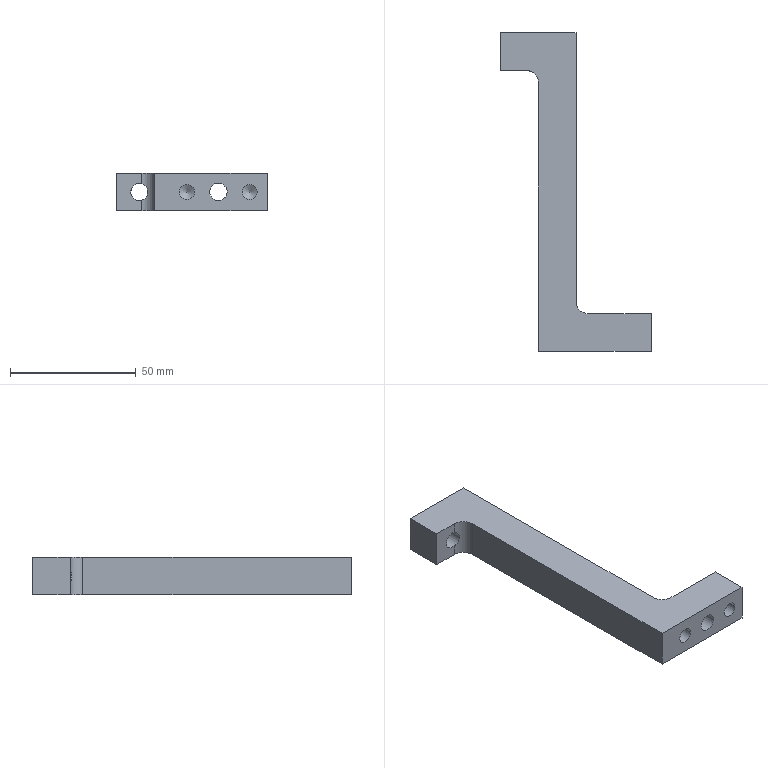Part | NX | features BREP 1 | 1 solid | 18 faces | box 60 x 127 x 15 mm | volume 37025 mm3 | plane 10 | cylinder 6 | cone 2 | commonest cylinder face diameters 6 x2 10 x2 6.8 x1 7 x1
STEP:
#1=CARTESIAN_POINT('',(14.,0.,7.5));
#2=VERTEX_POINT('',#1);
#3=CARTESIAN_POINT('',(10.5,0.,7.5));
#4=DIRECTION('',(0.,-1.,0.));
#5=DIRECTION('',(1.,0.,0.));
#6=AXIS2_PLACEMENT_3D('',#3,#4,#5);
#7=CIRCLE('',#6,3.5);
#8=EDGE_CURVE('',#2,#2,#7,.T.);
#9=ORIENTED_EDGE('',*,*,#8,.T.);
#10=EDGE_LOOP('',(#9));
#11=FACE_BOUND('',#10,.T.);
#12=CARTESIAN_POINT('',(30.,0.,0.));
#13=VERTEX_POINT('',#12);
#14=CARTESIAN_POINT('',(5.,0.,0.));
#15=VERTEX_POINT('',#14);
#16=CARTESIAN_POINT('',(30.,0.,0.));
#17=DIRECTION('',(-1.,0.,0.));
#18=VECTOR('',#17,1000.);
#19=LINE('',#16,#18);
#20=EDGE_CURVE('',#13,#15,#19,.T.);
#21=ORIENTED_EDGE('',*,*,#20,.T.);
#22=CARTESIAN_POINT('',(5.,0.,15.));
#23=VERTEX_POINT('',#22);
#24=CARTESIAN_POINT('',(5.,0.,15.));
#25=DIRECTION('',(0.,0.,1.));
#26=VECTOR('',#25,1000.);
#27=LINE('',#24,#26);
#28=EDGE_CURVE('',#15,#23,#27,.T.);
#29=ORIENTED_EDGE('',*,*,#28,.T.);
#30=CARTESIAN_POINT('',(30.,0.,15.));
#31=VERTEX_POINT('',#30);
#32=CARTESIAN_POINT('',(30.,0.,15.));
#33=DIRECTION('',(-1.,0.,0.));
#34=VECTOR('',#33,1000.);
#35=LINE('',#32,#34);
#36=EDGE_CURVE('',#31,#23,#35,.T.);
#37=ORIENTED_EDGE('',*,*,#36,.F.);
#38=CARTESIAN_POINT('',(30.,0.,15.));
#39=DIRECTION('',(0.,0.,-1.));
#40=VECTOR('',#39,1000.);
#41=LINE('',#38,#40);
#42=EDGE_CURVE('',#31,#13,#41,.T.);
#43=ORIENTED_EDGE('',*,*,#42,.T.);
#44=EDGE_LOOP('',(#21,#29,#37,#43));
#45=FACE_BOUND('',#44,.T.);
#46=CARTESIAN_POINT('',(30.,0.,15.));
#47=DIRECTION('',(0.,-1.,0.));
#48=DIRECTION('',(-1.,0.,0.));
#49=AXIS2_PLACEMENT_3D('',#46,#47,#48);
#50=PLANE('',#49);
#51=ADVANCED_FACE('',(#11,#45),#50,.F.);
#52=CARTESIAN_POINT('',(0.,5.,15.));
#53=VERTEX_POINT('',#52);
#54=CARTESIAN_POINT('',(0.,112.,15.));
#55=VERTEX_POINT('',#54);
#56=CARTESIAN_POINT('',(0.,0.,15.));
#57=DIRECTION('',(0.,1.,0.));
#58=VECTOR('',#57,1000.);
#59=LINE('',#56,#58);
#60=EDGE_CURVE('',#53,#55,#59,.T.);
#61=ORIENTED_EDGE('',*,*,#60,.F.);
#62=CARTESIAN_POINT('',(0.,5.,0.));
#63=VERTEX_POINT('',#62);
#64=CARTESIAN_POINT('',(0.,5.,0.));
#65=DIRECTION('',(0.,0.,-1.));
#66=VECTOR('',#65,1000.);
#67=LINE('',#64,#66);
#68=EDGE_CURVE('',#53,#63,#67,.T.);
#69=ORIENTED_EDGE('',*,*,#68,.T.);
#70=CARTESIAN_POINT('',(0.,112.,0.));
#71=VERTEX_POINT('',#70);
#72=CARTESIAN_POINT('',(0.,0.,0.));
#73=DIRECTION('',(0.,1.,0.));
#74=VECTOR('',#73,1000.);
#75=LINE('',#72,#74);
#76=EDGE_CURVE('',#63,#71,#75,.T.);
#77=ORIENTED_EDGE('',*,*,#76,.T.);
#78=CARTESIAN_POINT('',(0.,112.,15.));
#79=DIRECTION('',(0.,0.,-1.));
#80=VECTOR('',#79,1000.);
#81=LINE('',#78,#80);
#82=EDGE_CURVE('',#55,#71,#81,.T.);
#83=ORIENTED_EDGE('',*,*,#82,.F.);
#84=EDGE_LOOP('',(#61,#69,#77,#83));
#85=FACE_BOUND('',#84,.T.);
#86=CARTESIAN_POINT('',(0.,0.,15.));
#87=DIRECTION('',(-1.,0.,0.));
#88=DIRECTION('',(0.,1.,0.));
#89=AXIS2_PLACEMENT_3D('',#86,#87,#88);
#90=PLANE('',#89);
#91=ADVANCED_FACE('',(#85),#90,.F.);
#92=CARTESIAN_POINT('',(-21.,112.,10.9));
#93=VERTEX_POINT('',#92);
#94=CARTESIAN_POINT('',(-21.,112.,7.5));
#95=DIRECTION('',(0.,1.,0.));
#96=DIRECTION('',(0.,0.,1.));
#97=AXIS2_PLACEMENT_3D('',#94,#95,#96);
#98=CIRCLE('',#97,3.4);
#99=EDGE_CURVE('',#93,#93,#98,.T.);
#100=ORIENTED_EDGE('',*,*,#99,.F.);
#101=EDGE_LOOP('',(#100));
#102=FACE_BOUND('',#101,.T.);
#103=CARTESIAN_POINT('',(-30.,112.,0.));
#104=VERTEX_POINT('',#103);
#105=CARTESIAN_POINT('',(0.,112.,0.));
#106=DIRECTION('',(-1.,0.,0.));
#107=VECTOR('',#106,1000.);
#108=LINE('',#105,#107);
#109=EDGE_CURVE('',#71,#104,#108,.T.);
#110=ORIENTED_EDGE('',*,*,#109,.T.);
#111=CARTESIAN_POINT('',(-30.,112.,15.));
#112=VERTEX_POINT('',#111);
#113=CARTESIAN_POINT('',(-30.,112.,15.));
#114=DIRECTION('',(0.,0.,-1.));
#115=VECTOR('',#114,1000.);
#116=LINE('',#113,#115);
#117=EDGE_CURVE('',#112,#104,#116,.T.);
#118=ORIENTED_EDGE('',*,*,#117,.F.);
#119=CARTESIAN_POINT('',(0.,112.,15.));
#120=DIRECTION('',(-1.,0.,0.));
#121=VECTOR('',#120,1000.);
#122=LINE('',#119,#121);
#123=EDGE_CURVE('',#55,#112,#122,.T.);
#124=ORIENTED_EDGE('',*,*,#123,.F.);
#125=ORIENTED_EDGE('',*,*,#82,.T.);
#126=EDGE_LOOP('',(#110,#118,#124,#125));
#127=FACE_BOUND('',#126,.T.);
#128=CARTESIAN_POINT('',(0.,112.,15.));
#129=DIRECTION('',(0.,-1.,0.));
#130=DIRECTION('',(-1.,0.,0.));
#131=AXIS2_PLACEMENT_3D('',#128,#129,#130);
#132=PLANE('',#131);
#133=ADVANCED_FACE('',(#102,#127),#132,.F.);
#134=CARTESIAN_POINT('',(-30.,97.,0.));
#135=VERTEX_POINT('',#134);
#136=CARTESIAN_POINT('',(-30.,112.,0.));
#137=DIRECTION('',(0.,-1.,0.));
#138=VECTOR('',#137,1000.);
#139=LINE('',#136,#138);
#140=EDGE_CURVE('',#104,#135,#139,.T.);
#141=ORIENTED_EDGE('',*,*,#140,.T.);
#142=CARTESIAN_POINT('',(-30.,97.,15.));
#143=VERTEX_POINT('',#142);
#144=CARTESIAN_POINT('',(-30.,97.,15.));
#145=DIRECTION('',(0.,0.,-1.));
#146=VECTOR('',#145,1000.);
#147=LINE('',#144,#146);
#148=EDGE_CURVE('',#143,#135,#147,.T.);
#149=ORIENTED_EDGE('',*,*,#148,.F.);
#150=CARTESIAN_POINT('',(-30.,112.,15.));
#151=DIRECTION('',(0.,-1.,0.));
#152=VECTOR('',#151,1000.);
#153=LINE('',#150,#152);
#154=EDGE_CURVE('',#112,#143,#153,.T.);
#155=ORIENTED_EDGE('',*,*,#154,.F.);
#156=ORIENTED_EDGE('',*,*,#117,.T.);
#157=EDGE_LOOP('',(#141,#149,#155,#156));
#158=FACE_BOUND('',#157,.T.);
#159=CARTESIAN_POINT('',(-30.,112.,15.));
#160=DIRECTION('',(1.,0.,0.));
#161=DIRECTION('',(0.,-1.,0.));
#162=AXIS2_PLACEMENT_3D('',#159,#160,#161);
#163=PLANE('',#162);
#164=ADVANCED_FACE('',(#158),#163,.F.);
#165=CARTESIAN_POINT('',(-20.,97.,0.));
#166=VERTEX_POINT('',#165);
#167=CARTESIAN_POINT('',(-20.,97.,4.25));
#168=VERTEX_POINT('',#167);
#169=CARTESIAN_POINT('',(-20.,97.,15.));
#170=DIRECTION('',(0.,0.,1.));
#171=VECTOR('',#170,1000.);
#172=LINE('',#169,#171);
#173=EDGE_CURVE('',#166,#168,#172,.T.);
#174=ORIENTED_EDGE('',*,*,#173,.T.);
#175=CARTESIAN_POINT('',(-20.,97.,10.75));
#176=VERTEX_POINT('',#175);
#177=CARTESIAN_POINT('',(-21.,97.,7.5));
#178=DIRECTION('',(0.,1.,0.));
#179=DIRECTION('',(0.,0.,1.));
#180=AXIS2_PLACEMENT_3D('',#177,#178,#179);
#181=CIRCLE('',#180,3.4);
#182=EDGE_CURVE('',#168,#176,#181,.T.);
#183=ORIENTED_EDGE('',*,*,#182,.T.);
#184=CARTESIAN_POINT('',(-20.,97.,15.));
#185=VERTEX_POINT('',#184);
#186=CARTESIAN_POINT('',(-20.,97.,15.));
#187=DIRECTION('',(0.,0.,1.));
#188=VECTOR('',#187,1000.);
#189=LINE('',#186,#188);
#190=EDGE_CURVE('',#176,#185,#189,.T.);
#191=ORIENTED_EDGE('',*,*,#190,.T.);
#192=CARTESIAN_POINT('',(-30.,97.,15.));
#193=DIRECTION('',(1.,0.,0.));
#194=VECTOR('',#193,1000.);
#195=LINE('',#192,#194);
#196=EDGE_CURVE('',#143,#185,#195,.T.);
#197=ORIENTED_EDGE('',*,*,#196,.F.);
#198=ORIENTED_EDGE('',*,*,#148,.T.);
#199=CARTESIAN_POINT('',(-30.,97.,0.));
#200=DIRECTION('',(1.,0.,0.));
#201=VECTOR('',#200,1000.);
#202=LINE('',#199,#201);
#203=EDGE_CURVE('',#135,#166,#202,.T.);
#204=ORIENTED_EDGE('',*,*,#203,.T.);
#205=EDGE_LOOP('',(#174,#183,#191,#197,#198,#204));
#206=FACE_BOUND('',#205,.T.);
#207=CARTESIAN_POINT('',(-30.,97.,15.));
#208=DIRECTION('',(0.,1.,0.));
#209=DIRECTION('',(0.,0.,-1.));
#210=AXIS2_PLACEMENT_3D('',#207,#208,#209);
#211=PLANE('',#210);
#212=ADVANCED_FACE('',(#206),#211,.F.);
#213=CARTESIAN_POINT('',(-15.,92.,15.));
#214=VERTEX_POINT('',#213);
#215=CARTESIAN_POINT('',(-15.,-15.,15.));
#216=VERTEX_POINT('',#215);
#217=CARTESIAN_POINT('',(-15.,97.,15.));
#218=DIRECTION('',(0.,-1.,0.));
#219=VECTOR('',#218,1000.);
#220=LINE('',#217,#219);
#221=EDGE_CURVE('',#214,#216,#220,.T.);
#222=ORIENTED_EDGE('',*,*,#221,.F.);
#223=CARTESIAN_POINT('',(-15.,92.,0.));
#224=VERTEX_POINT('',#223);
#225=CARTESIAN_POINT('',(-15.,92.,0.));
#226=DIRECTION('',(0.,0.,-1.));
#227=VECTOR('',#226,1000.);
#228=LINE('',#225,#227);
#229=EDGE_CURVE('',#214,#224,#228,.T.);
#230=ORIENTED_EDGE('',*,*,#229,.T.);
#231=CARTESIAN_POINT('',(-15.,-15.,0.));
#232=VERTEX_POINT('',#231);
#233=CARTESIAN_POINT('',(-15.,97.,0.));
#234=DIRECTION('',(0.,-1.,0.));
#235=VECTOR('',#234,1000.);
#236=LINE('',#233,#235);
#237=EDGE_CURVE('',#224,#232,#236,.T.);
#238=ORIENTED_EDGE('',*,*,#237,.T.);
#239=CARTESIAN_POINT('',(-15.,-15.,15.));
#240=DIRECTION('',(0.,0.,-1.));
#241=VECTOR('',#240,1000.);
#242=LINE('',#239,#241);
#243=EDGE_CURVE('',#216,#232,#242,.T.);
#244=ORIENTED_EDGE('',*,*,#243,.F.);
#245=EDGE_LOOP('',(#222,#230,#238,#244));
#246=FACE_BOUND('',#245,.T.);
#247=CARTESIAN_POINT('',(-15.,97.,15.));
#248=DIRECTION('',(1.,0.,0.));
#249=DIRECTION('',(0.,-1.,0.));
#250=AXIS2_PLACEMENT_3D('',#247,#248,#249);
#251=PLANE('',#250);
#252=ADVANCED_FACE('',(#246),#251,.F.);
#253=CARTESIAN_POINT('',(10.5,-15.,4.));
#254=VERTEX_POINT('',#253);
#255=CARTESIAN_POINT('',(10.5,-15.,7.5));
#256=DIRECTION('',(0.,-1.,0.));
#257=DIRECTION('',(0.,0.,-1.));
#258=AXIS2_PLACEMENT_3D('',#255,#256,#257);
#259=CIRCLE('',#258,3.5);
#260=EDGE_CURVE('',#254,#254,#259,.T.);
#261=ORIENTED_EDGE('',*,*,#260,.F.);
#262=EDGE_LOOP('',(#261));
#263=FACE_BOUND('',#262,.T.);
#264=CARTESIAN_POINT('',(23.,-15.,4.5));
#265=VERTEX_POINT('',#264);
#266=CARTESIAN_POINT('',(23.,-15.,7.5));
#267=DIRECTION('',(0.,-1.,0.));
#268=DIRECTION('',(0.,0.,-1.));
#269=AXIS2_PLACEMENT_3D('',#266,#267,#268);
#270=CIRCLE('',#269,3.);
#271=EDGE_CURVE('',#265,#265,#270,.T.);
#272=ORIENTED_EDGE('',*,*,#271,.F.);
#273=EDGE_LOOP('',(#272));
#274=FACE_BOUND('',#273,.T.);
#275=CARTESIAN_POINT('',(-2.,-15.,4.5));
#276=VERTEX_POINT('',#275);
#277=CARTESIAN_POINT('',(-2.,-15.,7.5));
#278=DIRECTION('',(0.,-1.,0.));
#279=DIRECTION('',(0.,0.,-1.));
#280=AXIS2_PLACEMENT_3D('',#277,#278,#279);
#281=CIRCLE('',#280,3.);
#282=EDGE_CURVE('',#276,#276,#281,.T.);
#283=ORIENTED_EDGE('',*,*,#282,.F.);
#284=EDGE_LOOP('',(#283));
#285=FACE_BOUND('',#284,.T.);
#286=CARTESIAN_POINT('',(30.,-15.,0.));
#287=VERTEX_POINT('',#286);
#288=CARTESIAN_POINT('',(-15.,-15.,0.));
#289=DIRECTION('',(1.,0.,0.));
#290=VECTOR('',#289,1000.);
#291=LINE('',#288,#290);
#292=EDGE_CURVE('',#232,#287,#291,.T.);
#293=ORIENTED_EDGE('',*,*,#292,.T.);
#294=CARTESIAN_POINT('',(30.,-15.,15.));
#295=VERTEX_POINT('',#294);
#296=CARTESIAN_POINT('',(30.,-15.,15.));
#297=DIRECTION('',(0.,0.,-1.));
#298=VECTOR('',#297,1000.);
#299=LINE('',#296,#298);
#300=EDGE_CURVE('',#295,#287,#299,.T.);
#301=ORIENTED_EDGE('',*,*,#300,.F.);
#302=CARTESIAN_POINT('',(-15.,-15.,15.));
#303=DIRECTION('',(1.,0.,0.));
#304=VECTOR('',#303,1000.);
#305=LINE('',#302,#304);
#306=EDGE_CURVE('',#216,#295,#305,.T.);
#307=ORIENTED_EDGE('',*,*,#306,.F.);
#308=ORIENTED_EDGE('',*,*,#243,.T.);
#309=EDGE_LOOP('',(#293,#301,#307,#308));
#310=FACE_BOUND('',#309,.T.);
#311=CARTESIAN_POINT('',(-15.,-15.,15.));
#312=DIRECTION('',(0.,1.,0.));
#313=DIRECTION('',(0.,0.,-1.));
#314=AXIS2_PLACEMENT_3D('',#311,#312,#313);
#315=PLANE('',#314);
#316=ADVANCED_FACE('',(#263,#274,#285,#310),#315,.F.);
#317=CARTESIAN_POINT('',(30.,-15.,0.));
#318=DIRECTION('',(0.,1.,0.));
#319=VECTOR('',#318,1000.);
#320=LINE('',#317,#319);
#321=EDGE_CURVE('',#287,#13,#320,.T.);
#322=ORIENTED_EDGE('',*,*,#321,.T.);
#323=ORIENTED_EDGE('',*,*,#42,.F.);
#324=CARTESIAN_POINT('',(30.,-15.,15.));
#325=DIRECTION('',(0.,1.,0.));
#326=VECTOR('',#325,1000.);
#327=LINE('',#324,#326);
#328=EDGE_CURVE('',#295,#31,#327,.T.);
#329=ORIENTED_EDGE('',*,*,#328,.F.);
#330=ORIENTED_EDGE('',*,*,#300,.T.);
#331=EDGE_LOOP('',(#322,#323,#329,#330));
#332=FACE_BOUND('',#331,.T.);
#333=CARTESIAN_POINT('',(30.,-15.,15.));
#334=DIRECTION('',(-1.,0.,0.));
#335=DIRECTION('',(0.,0.,-1.));
#336=AXIS2_PLACEMENT_3D('',#333,#334,#335);
#337=PLANE('',#336);
#338=ADVANCED_FACE('',(#332),#337,.F.);
#339=ORIENTED_EDGE('',*,*,#36,.T.);
#340=CARTESIAN_POINT('',(5.,5.,15.));
#341=DIRECTION('',(0.,0.,-1.));
#342=DIRECTION('',(-1.,0.,0.));
#343=AXIS2_PLACEMENT_3D('',#340,#341,#342);
#344=CIRCLE('',#343,5.);
#345=EDGE_CURVE('',#23,#53,#344,.T.);
#346=ORIENTED_EDGE('',*,*,#345,.T.);
#347=ORIENTED_EDGE('',*,*,#60,.T.);
#348=ORIENTED_EDGE('',*,*,#123,.T.);
#349=ORIENTED_EDGE('',*,*,#154,.T.);
#350=ORIENTED_EDGE('',*,*,#196,.T.);
#351=CARTESIAN_POINT('',(-20.,92.,15.));
#352=DIRECTION('',(0.,0.,-1.));
#353=DIRECTION('',(-1.,0.,0.));
#354=AXIS2_PLACEMENT_3D('',#351,#352,#353);
#355=CIRCLE('',#354,5.);
#356=EDGE_CURVE('',#185,#214,#355,.T.);
#357=ORIENTED_EDGE('',*,*,#356,.T.);
#358=ORIENTED_EDGE('',*,*,#221,.T.);
#359=ORIENTED_EDGE('',*,*,#306,.T.);
#360=ORIENTED_EDGE('',*,*,#328,.T.);
#361=EDGE_LOOP('',(#339,#346,#347,#348,#349,#350,#357,#358,#359,#360));
#362=FACE_BOUND('',#361,.T.);
#363=CARTESIAN_POINT('',(0.,0.,15.));
#364=DIRECTION('',(0.,0.,-1.));
#365=DIRECTION('',(1.,0.,0.));
#366=AXIS2_PLACEMENT_3D('',#363,#364,#365);
#367=PLANE('',#366);
#368=ADVANCED_FACE('',(#362),#367,.F.);
#369=ORIENTED_EDGE('',*,*,#20,.F.);
#370=ORIENTED_EDGE('',*,*,#321,.F.);
#371=ORIENTED_EDGE('',*,*,#292,.F.);
#372=ORIENTED_EDGE('',*,*,#237,.F.);
#373=CARTESIAN_POINT('',(-20.,92.,0.));
#374=DIRECTION('',(0.,0.,1.));
#375=DIRECTION('',(-1.,0.,0.));
#376=AXIS2_PLACEMENT_3D('',#373,#374,#375);
#377=CIRCLE('',#376,5.);
#378=EDGE_CURVE('',#224,#166,#377,.T.);
#379=ORIENTED_EDGE('',*,*,#378,.T.);
#380=ORIENTED_EDGE('',*,*,#203,.F.);
#381=ORIENTED_EDGE('',*,*,#140,.F.);
#382=ORIENTED_EDGE('',*,*,#109,.F.);
#383=ORIENTED_EDGE('',*,*,#76,.F.);
#384=CARTESIAN_POINT('',(5.,5.,0.));
#385=DIRECTION('',(0.,0.,1.));
#386=DIRECTION('',(-1.,0.,0.));
#387=AXIS2_PLACEMENT_3D('',#384,#385,#386);
#388=CIRCLE('',#387,5.);
#389=EDGE_CURVE('',#63,#15,#388,.T.);
#390=ORIENTED_EDGE('',*,*,#389,.T.);
#391=EDGE_LOOP('',(#369,#370,#371,#372,#379,#380,#381,#382,#383,#390));
#392=FACE_BOUND('',#391,.T.);
#393=CARTESIAN_POINT('',(0.,0.,0.));
#394=DIRECTION('',(0.,0.,-1.));
#395=DIRECTION('',(1.,0.,0.));
#396=AXIS2_PLACEMENT_3D('',#393,#394,#395);
#397=PLANE('',#396);
#398=ADVANCED_FACE('',(#392),#397,.T.);
#399=ORIENTED_EDGE('',*,*,#345,.F.);
#400=ORIENTED_EDGE('',*,*,#28,.F.);
#401=ORIENTED_EDGE('',*,*,#389,.F.);
#402=ORIENTED_EDGE('',*,*,#68,.F.);
#403=EDGE_LOOP('',(#399,#400,#401,#402));
#404=FACE_BOUND('',#403,.T.);
#405=CARTESIAN_POINT('',(5.,5.,15.));
#406=DIRECTION('',(0.,0.,1.));
#407=DIRECTION('',(-1.,0.,0.));
#408=AXIS2_PLACEMENT_3D('',#405,#406,#407);
#409=CYLINDRICAL_SURFACE('',#408,5.);
#410=ADVANCED_FACE('',(#404),#409,.F.);
#411=ORIENTED_EDGE('',*,*,#190,.F.);
#412=CARTESIAN_POINT('',(-20.,97.,10.75));
#413=CARTESIAN_POINT('',(-19.295,97.,10.533));
#414=CARTESIAN_POINT('',(-18.083,96.686,9.661));
#415=CARTESIAN_POINT('',(-17.359,96.237,7.507));
#416=CARTESIAN_POINT('',(-18.082,96.685,5.336));
#417=CARTESIAN_POINT('',(-19.295,97.,4.467));
#418=CARTESIAN_POINT('',(-20.,97.,4.25));
#419=B_SPLINE_CURVE_WITH_KNOTS('',3,(#412,#413,#414,#415,#416,#417,#418),.UNSPECIFIED.,.F.,.F.,(4,1,1,1,4),(0.,0.002177,0.004353,0.00653,0.008706),.UNSPECIFIED.);
#420=EDGE_CURVE('',#176,#168,#419,.T.);
#421=ORIENTED_EDGE('',*,*,#420,.T.);
#422=ORIENTED_EDGE('',*,*,#173,.F.);
#423=ORIENTED_EDGE('',*,*,#378,.F.);
#424=ORIENTED_EDGE('',*,*,#229,.F.);
#425=ORIENTED_EDGE('',*,*,#356,.F.);
#426=EDGE_LOOP('',(#411,#421,#422,#423,#424,#425));
#427=FACE_BOUND('',#426,.T.);
#428=CARTESIAN_POINT('',(-20.,92.,15.));
#429=DIRECTION('',(0.,0.,1.));
#430=DIRECTION('',(-1.,0.,0.));
#431=AXIS2_PLACEMENT_3D('',#428,#429,#430);
#432=CYLINDRICAL_SURFACE('',#431,5.);
#433=ADVANCED_FACE('',(#427),#432,.F.);
#434=ORIENTED_EDGE('',*,*,#99,.T.);
#435=EDGE_LOOP('',(#434));
#436=FACE_BOUND('',#435,.T.);
#437=ORIENTED_EDGE('',*,*,#420,.F.);
#438=ORIENTED_EDGE('',*,*,#182,.F.);
#439=EDGE_LOOP('',(#437,#438));
#440=FACE_BOUND('',#439,.T.);
#441=CARTESIAN_POINT('',(-21.,112.,7.5));
#442=DIRECTION('',(0.,1.,0.));
#443=DIRECTION('',(0.,0.,-1.));
#444=AXIS2_PLACEMENT_3D('',#441,#442,#443);
#445=CYLINDRICAL_SURFACE('',#444,3.4);
#446=ADVANCED_FACE('',(#436,#440),#445,.F.);
#447=CARTESIAN_POINT('',(-2.,-1.197,7.5));
#448=VERTEX_POINT('',#447);
#449=VERTEX_LOOP('',#448);
#450=FACE_BOUND('',#449,.T.);
#451=CARTESIAN_POINT('',(-2.,-3.,4.5));
#452=VERTEX_POINT('',#451);
#453=CARTESIAN_POINT('',(-2.,-3.,7.5));
#454=DIRECTION('',(0.,-1.,0.));
#455=DIRECTION('',(0.,0.,-1.));
#456=AXIS2_PLACEMENT_3D('',#453,#454,#455);
#457=CIRCLE('',#456,3.);
#458=EDGE_CURVE('',#452,#452,#457,.T.);
#459=ORIENTED_EDGE('',*,*,#458,.T.);
#460=EDGE_LOOP('',(#459));
#461=FACE_BOUND('',#460,.T.);
#462=CARTESIAN_POINT('',(-2.,-3.,7.5));
#463=DIRECTION('',(0.,-1.,0.));
#464=DIRECTION('',(0.,0.,1.));
#465=AXIS2_PLACEMENT_3D('',#462,#463,#464);
#466=CONICAL_SURFACE('',#465,3.,1.03);
#467=ADVANCED_FACE('',(#450,#461),#466,.F.);
#468=ORIENTED_EDGE('',*,*,#458,.F.);
#469=EDGE_LOOP('',(#468));
#470=FACE_BOUND('',#469,.T.);
#471=ORIENTED_EDGE('',*,*,#282,.T.);
#472=EDGE_LOOP('',(#471));
#473=FACE_BOUND('',#472,.T.);
#474=CARTESIAN_POINT('',(-2.,-15.,7.5));
#475=DIRECTION('',(0.,-1.,0.));
#476=DIRECTION('',(0.,0.,1.));
#477=AXIS2_PLACEMENT_3D('',#474,#475,#476);
#478=CYLINDRICAL_SURFACE('',#477,3.);
#479=ADVANCED_FACE('',(#470,#473),#478,.F.);
#480=CARTESIAN_POINT('',(23.,-1.197,7.5));
#481=VERTEX_POINT('',#480);
#482=VERTEX_LOOP('',#481);
#483=FACE_BOUND('',#482,.T.);
#484=CARTESIAN_POINT('',(23.,-3.,4.5));
#485=VERTEX_POINT('',#484);
#486=CARTESIAN_POINT('',(23.,-3.,7.5));
#487=DIRECTION('',(0.,-1.,0.));
#488=DIRECTION('',(0.,0.,-1.));
#489=AXIS2_PLACEMENT_3D('',#486,#487,#488);
#490=CIRCLE('',#489,3.);
#491=EDGE_CURVE('',#485,#485,#490,.T.);
#492=ORIENTED_EDGE('',*,*,#491,.T.);
#493=EDGE_LOOP('',(#492));
#494=FACE_BOUND('',#493,.T.);
#495=CARTESIAN_POINT('',(23.,-3.,7.5));
#496=DIRECTION('',(0.,-1.,0.));
#497=DIRECTION('',(0.,0.,1.));
#498=AXIS2_PLACEMENT_3D('',#495,#496,#497);
#499=CONICAL_SURFACE('',#498,3.,1.03);
#500=ADVANCED_FACE('',(#483,#494),#499,.F.);
#501=ORIENTED_EDGE('',*,*,#491,.F.);
#502=EDGE_LOOP('',(#501));
#503=FACE_BOUND('',#502,.T.);
#504=ORIENTED_EDGE('',*,*,#271,.T.);
#505=EDGE_LOOP('',(#504));
#506=FACE_BOUND('',#505,.T.);
#507=CARTESIAN_POINT('',(23.,-15.,7.5));
#508=DIRECTION('',(0.,-1.,0.));
#509=DIRECTION('',(0.,0.,1.));
#510=AXIS2_PLACEMENT_3D('',#507,#508,#509);
#511=CYLINDRICAL_SURFACE('',#510,3.);
#512=ADVANCED_FACE('',(#503,#506),#511,.F.);
#513=ORIENTED_EDGE('',*,*,#260,.T.);
#514=EDGE_LOOP('',(#513));
#515=FACE_BOUND('',#514,.T.);
#516=ORIENTED_EDGE('',*,*,#8,.F.);
#517=EDGE_LOOP('',(#516));
#518=FACE_BOUND('',#517,.T.);
#519=CARTESIAN_POINT('',(10.5,-15.,7.5));
#520=DIRECTION('',(0.,-1.,0.));
#521=DIRECTION('',(0.,0.,1.));
#522=AXIS2_PLACEMENT_3D('',#519,#520,#521);
#523=CYLINDRICAL_SURFACE('',#522,3.5);
#524=ADVANCED_FACE('',(#515,#518),#523,.F.);
#525=CLOSED_SHELL('',(#51,#91,#133,#164,#212,#252,#316,#338,#368,#398,#410,#433,#446,#467,#479,#500,#512,#524));
#526=MANIFOLD_SOLID_BREP('',#525);
#527=(LENGTH_UNIT()NAMED_UNIT(*)SI_UNIT(.MILLI.,.METRE.));
#528=UNCERTAINTY_MEASURE_WITH_UNIT(LENGTH_MEASURE(0.0508),#527,'','');
#529=(NAMED_UNIT(*)PLANE_ANGLE_UNIT()SI_UNIT($,.RADIAN.));
#530=(NAMED_UNIT(*)SI_UNIT($,.STERADIAN.)SOLID_ANGLE_UNIT());
#531=(GEOMETRIC_REPRESENTATION_CONTEXT(3)GLOBAL_UNCERTAINTY_ASSIGNED_CONTEXT((#528))GLOBAL_UNIT_ASSIGNED_CONTEXT((#527,#529,#530))REPRESENTATION_CONTEXT('',''));
#532=ADVANCED_BREP_SHAPE_REPRESENTATION('',(#526),#531);